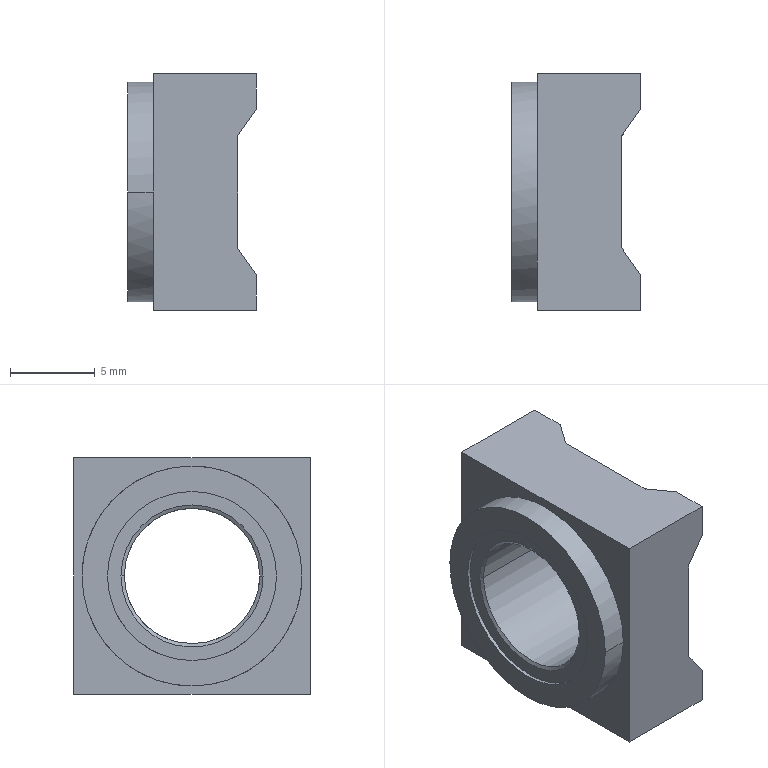Part | NX | features BREP 1 | 1 solid | 28 faces | box 7.6 x 14 x 14 mm | volume 863.218 mm3 | plane 16 | cylinder 6 | cone 6 | commonest cylinder face diameters 8 x2 10 x2 13 x2